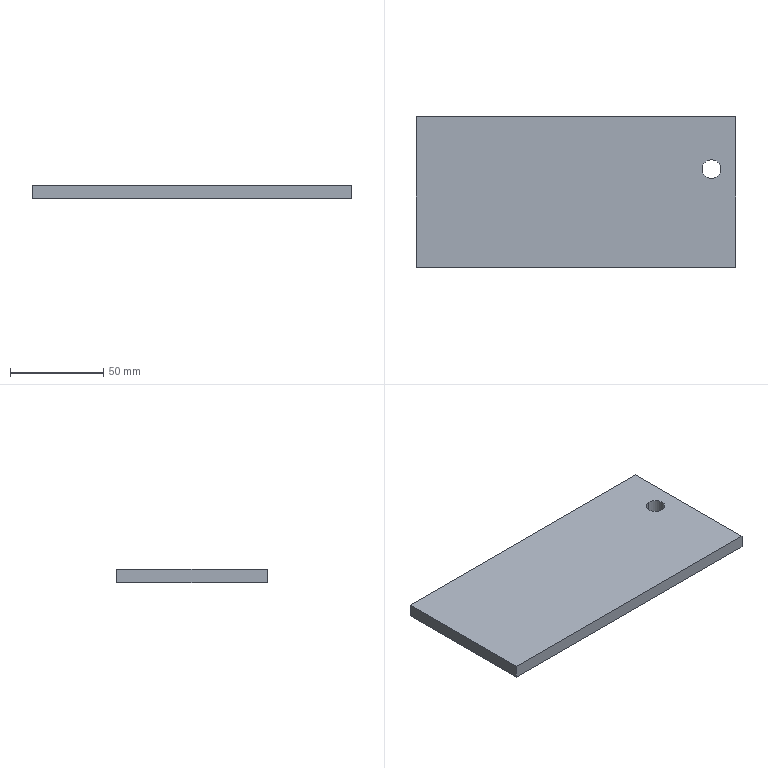Part | STEP file | 2026.6.15-Main Assembly图.sldasm-Part-138 | 1 solid | 8 faces | box 170.9 x 80.5 x 7 mm | volume 95752 mm3 | plane 6 | cylinder 2 | commonest cylinder face diameters 10 x2
STEP:
#1=CARTESIAN_POINT('',(-1516.724,576.551,4343.667));
#2=VERTEX_POINT('',#1);
#3=CARTESIAN_POINT('',(-1516.724,566.551,4343.667));
#4=VERTEX_POINT('',#3);
#5=CARTESIAN_POINT('',(-1516.724,571.551,4343.667));
#6=DIRECTION('',(0.,0.,1.));
#7=DIRECTION('',(0.,-1.,0.));
#8=AXIS2_PLACEMENT_3D('',#5,#6,#7);
#9=CIRCLE('',#8,5.);
#10=EDGE_CURVE('',#2,#4,#9,.T.);
#11=ORIENTED_EDGE('',*,*,#10,.T.);
#12=CARTESIAN_POINT('',(-1516.724,566.551,4336.667));
#13=VERTEX_POINT('',#12);
#14=CARTESIAN_POINT('',(-1516.724,566.551,4343.667));
#15=DIRECTION('',(0.,0.,-1.));
#16=VECTOR('',#15,1000.);
#17=LINE('',#14,#16);
#18=EDGE_CURVE('',#4,#13,#17,.T.);
#19=ORIENTED_EDGE('',*,*,#18,.T.);
#20=CARTESIAN_POINT('',(-1516.724,576.551,4336.667));
#21=VERTEX_POINT('',#20);
#22=CARTESIAN_POINT('',(-1516.724,571.551,4336.667));
#23=DIRECTION('',(0.,0.,1.));
#24=DIRECTION('',(0.,-1.,0.));
#25=AXIS2_PLACEMENT_3D('',#22,#23,#24);
#26=CIRCLE('',#25,5.);
#27=EDGE_CURVE('',#21,#13,#26,.T.);
#28=ORIENTED_EDGE('',*,*,#27,.F.);
#29=CARTESIAN_POINT('',(-1516.724,576.551,4343.667));
#30=DIRECTION('',(0.,0.,-1.));
#31=VECTOR('',#30,1000.);
#32=LINE('',#29,#31);
#33=EDGE_CURVE('',#2,#21,#32,.T.);
#34=ORIENTED_EDGE('',*,*,#33,.F.);
#35=EDGE_LOOP('',(#11,#19,#28,#34));
#36=FACE_OUTER_BOUND('',#35,.T.);
#37=CARTESIAN_POINT('',(-1516.724,571.551,4343.667));
#38=DIRECTION('',(0.,0.,-1.));
#39=DIRECTION('',(0.,1.,0.));
#40=AXIS2_PLACEMENT_3D('',#37,#38,#39);
#41=CYLINDRICAL_SURFACE('',#40,5.);
#42=ADVANCED_FACE('',(#36),#41,.F.);
#43=CARTESIAN_POINT('',(-1674.674,599.551,4336.667));
#44=VERTEX_POINT('',#43);
#45=CARTESIAN_POINT('',(-1674.674,519.051,4336.667));
#46=VERTEX_POINT('',#45);
#47=CARTESIAN_POINT('',(-1674.674,599.551,4336.667));
#48=DIRECTION('',(0.,-1.,0.));
#49=VECTOR('',#48,1000.);
#50=LINE('',#47,#49);
#51=EDGE_CURVE('',#44,#46,#50,.T.);
#52=ORIENTED_EDGE('',*,*,#51,.T.);
#53=CARTESIAN_POINT('',(-1674.674,519.051,4343.667));
#54=VERTEX_POINT('',#53);
#55=CARTESIAN_POINT('',(-1674.674,519.051,4343.667));
#56=DIRECTION('',(0.,0.,-1.));
#57=VECTOR('',#56,1000.);
#58=LINE('',#55,#57);
#59=EDGE_CURVE('',#54,#46,#58,.T.);
#60=ORIENTED_EDGE('',*,*,#59,.F.);
#61=CARTESIAN_POINT('',(-1674.674,599.551,4343.667));
#62=VERTEX_POINT('',#61);
#63=CARTESIAN_POINT('',(-1674.674,599.551,4343.667));
#64=DIRECTION('',(0.,-1.,0.));
#65=VECTOR('',#64,1000.);
#66=LINE('',#63,#65);
#67=EDGE_CURVE('',#62,#54,#66,.T.);
#68=ORIENTED_EDGE('',*,*,#67,.F.);
#69=CARTESIAN_POINT('',(-1674.674,599.551,4343.667));
#70=DIRECTION('',(0.,0.,-1.));
#71=VECTOR('',#70,1000.);
#72=LINE('',#69,#71);
#73=EDGE_CURVE('',#62,#44,#72,.T.);
#74=ORIENTED_EDGE('',*,*,#73,.T.);
#75=EDGE_LOOP('',(#52,#60,#68,#74));
#76=FACE_OUTER_BOUND('',#75,.T.);
#77=CARTESIAN_POINT('',(-1674.674,599.551,4343.667));
#78=DIRECTION('',(1.,0.,0.));
#79=DIRECTION('',(0.,1.,0.));
#80=AXIS2_PLACEMENT_3D('',#77,#78,#79);
#81=PLANE('',#80);
#82=ADVANCED_FACE('',(#76),#81,.F.);
#83=CARTESIAN_POINT('',(-1503.774,519.051,4336.667));
#84=VERTEX_POINT('',#83);
#85=CARTESIAN_POINT('',(-1674.674,519.051,4336.667));
#86=DIRECTION('',(1.,0.,0.));
#87=VECTOR('',#86,1000.);
#88=LINE('',#85,#87);
#89=EDGE_CURVE('',#46,#84,#88,.T.);
#90=ORIENTED_EDGE('',*,*,#89,.T.);
#91=CARTESIAN_POINT('',(-1503.774,519.051,4343.667));
#92=VERTEX_POINT('',#91);
#93=CARTESIAN_POINT('',(-1503.774,519.051,4343.667));
#94=DIRECTION('',(0.,0.,-1.));
#95=VECTOR('',#94,1000.);
#96=LINE('',#93,#95);
#97=EDGE_CURVE('',#92,#84,#96,.T.);
#98=ORIENTED_EDGE('',*,*,#97,.F.);
#99=CARTESIAN_POINT('',(-1674.674,519.051,4343.667));
#100=DIRECTION('',(1.,0.,0.));
#101=VECTOR('',#100,1000.);
#102=LINE('',#99,#101);
#103=EDGE_CURVE('',#54,#92,#102,.T.);
#104=ORIENTED_EDGE('',*,*,#103,.F.);
#105=ORIENTED_EDGE('',*,*,#59,.T.);
#106=EDGE_LOOP('',(#90,#98,#104,#105));
#107=FACE_OUTER_BOUND('',#106,.T.);
#108=CARTESIAN_POINT('',(-1674.674,519.051,4343.667));
#109=DIRECTION('',(0.,1.,0.));
#110=DIRECTION('',(0.,0.,1.));
#111=AXIS2_PLACEMENT_3D('',#108,#109,#110);
#112=PLANE('',#111);
#113=ADVANCED_FACE('',(#107),#112,.F.);
#114=CARTESIAN_POINT('',(-1503.774,599.551,4336.667));
#115=VERTEX_POINT('',#114);
#116=CARTESIAN_POINT('',(-1503.774,519.051,4336.667));
#117=DIRECTION('',(0.,1.,0.));
#118=VECTOR('',#117,1000.);
#119=LINE('',#116,#118);
#120=EDGE_CURVE('',#84,#115,#119,.T.);
#121=ORIENTED_EDGE('',*,*,#120,.T.);
#122=CARTESIAN_POINT('',(-1503.774,599.551,4343.667));
#123=VERTEX_POINT('',#122);
#124=CARTESIAN_POINT('',(-1503.774,599.551,4343.667));
#125=DIRECTION('',(0.,0.,-1.));
#126=VECTOR('',#125,1000.);
#127=LINE('',#124,#126);
#128=EDGE_CURVE('',#123,#115,#127,.T.);
#129=ORIENTED_EDGE('',*,*,#128,.F.);
#130=CARTESIAN_POINT('',(-1503.774,519.051,4343.667));
#131=DIRECTION('',(0.,1.,0.));
#132=VECTOR('',#131,1000.);
#133=LINE('',#130,#132);
#134=EDGE_CURVE('',#92,#123,#133,.T.);
#135=ORIENTED_EDGE('',*,*,#134,.F.);
#136=ORIENTED_EDGE('',*,*,#97,.T.);
#137=EDGE_LOOP('',(#121,#129,#135,#136));
#138=FACE_OUTER_BOUND('',#137,.T.);
#139=CARTESIAN_POINT('',(-1503.774,519.051,4343.667));
#140=DIRECTION('',(-1.,0.,0.));
#141=DIRECTION('',(0.,-1.,0.));
#142=AXIS2_PLACEMENT_3D('',#139,#140,#141);
#143=PLANE('',#142);
#144=ADVANCED_FACE('',(#138),#143,.F.);
#145=CARTESIAN_POINT('',(-1503.774,599.551,4336.667));
#146=DIRECTION('',(-1.,0.,0.));
#147=VECTOR('',#146,1000.);
#148=LINE('',#145,#147);
#149=EDGE_CURVE('',#115,#44,#148,.T.);
#150=ORIENTED_EDGE('',*,*,#149,.T.);
#151=ORIENTED_EDGE('',*,*,#73,.F.);
#152=CARTESIAN_POINT('',(-1503.774,599.551,4343.667));
#153=DIRECTION('',(-1.,0.,0.));
#154=VECTOR('',#153,1000.);
#155=LINE('',#152,#154);
#156=EDGE_CURVE('',#123,#62,#155,.T.);
#157=ORIENTED_EDGE('',*,*,#156,.F.);
#158=ORIENTED_EDGE('',*,*,#128,.T.);
#159=EDGE_LOOP('',(#150,#151,#157,#158));
#160=FACE_OUTER_BOUND('',#159,.T.);
#161=CARTESIAN_POINT('',(-1503.774,599.551,4343.667));
#162=DIRECTION('',(0.,-1.,0.));
#163=DIRECTION('',(0.,0.,-1.));
#164=AXIS2_PLACEMENT_3D('',#161,#162,#163);
#165=PLANE('',#164);
#166=ADVANCED_FACE('',(#160),#165,.F.);
#167=ORIENTED_EDGE('',*,*,#18,.F.);
#168=CARTESIAN_POINT('',(-1516.724,571.551,4343.667));
#169=DIRECTION('',(0.,0.,1.));
#170=DIRECTION('',(0.,-1.,0.));
#171=AXIS2_PLACEMENT_3D('',#168,#169,#170);
#172=CIRCLE('',#171,5.);
#173=EDGE_CURVE('',#4,#2,#172,.T.);
#174=ORIENTED_EDGE('',*,*,#173,.T.);
#175=ORIENTED_EDGE('',*,*,#33,.T.);
#176=CARTESIAN_POINT('',(-1516.724,571.551,4336.667));
#177=DIRECTION('',(0.,0.,1.));
#178=DIRECTION('',(0.,-1.,0.));
#179=AXIS2_PLACEMENT_3D('',#176,#177,#178);
#180=CIRCLE('',#179,5.);
#181=EDGE_CURVE('',#13,#21,#180,.T.);
#182=ORIENTED_EDGE('',*,*,#181,.F.);
#183=EDGE_LOOP('',(#167,#174,#175,#182));
#184=FACE_OUTER_BOUND('',#183,.T.);
#185=CARTESIAN_POINT('',(-1516.724,571.551,4343.667));
#186=DIRECTION('',(0.,0.,-1.));
#187=DIRECTION('',(0.,1.,0.));
#188=AXIS2_PLACEMENT_3D('',#185,#186,#187);
#189=CYLINDRICAL_SURFACE('',#188,5.);
#190=ADVANCED_FACE('',(#184),#189,.F.);
#191=ORIENTED_EDGE('',*,*,#67,.T.);
#192=ORIENTED_EDGE('',*,*,#103,.T.);
#193=ORIENTED_EDGE('',*,*,#134,.T.);
#194=ORIENTED_EDGE('',*,*,#156,.T.);
#195=EDGE_LOOP('',(#191,#192,#193,#194));
#196=FACE_OUTER_BOUND('',#195,.T.);
#197=ORIENTED_EDGE('',*,*,#10,.F.);
#198=ORIENTED_EDGE('',*,*,#173,.F.);
#199=EDGE_LOOP('',(#197,#198));
#200=FACE_BOUND('',#199,.T.);
#201=CARTESIAN_POINT('',(-1516.724,571.551,4343.667));
#202=DIRECTION('',(0.,0.,1.));
#203=DIRECTION('',(0.,-1.,0.));
#204=AXIS2_PLACEMENT_3D('',#201,#202,#203);
#205=PLANE('',#204);
#206=ADVANCED_FACE('',(#196,#200),#205,.T.);
#207=ORIENTED_EDGE('',*,*,#51,.F.);
#208=ORIENTED_EDGE('',*,*,#149,.F.);
#209=ORIENTED_EDGE('',*,*,#120,.F.);
#210=ORIENTED_EDGE('',*,*,#89,.F.);
#211=EDGE_LOOP('',(#207,#208,#209,#210));
#212=FACE_OUTER_BOUND('',#211,.T.);
#213=ORIENTED_EDGE('',*,*,#27,.T.);
#214=ORIENTED_EDGE('',*,*,#181,.T.);
#215=EDGE_LOOP('',(#213,#214));
#216=FACE_BOUND('',#215,.T.);
#217=CARTESIAN_POINT('',(-1516.724,571.551,4336.667));
#218=DIRECTION('',(0.,0.,1.));
#219=DIRECTION('',(0.,-1.,0.));
#220=AXIS2_PLACEMENT_3D('',#217,#218,#219);
#221=PLANE('',#220);
#222=ADVANCED_FACE('',(#212,#216),#221,.F.);
#223=CLOSED_SHELL('',(#42,#82,#113,#144,#166,#190,#206,#222));
#224=MANIFOLD_SOLID_BREP('',#223);
#225=CARTESIAN_POINT('',(0.,0.,0.));
#226=DIRECTION('',(0.,0.,1.));
#227=DIRECTION('',(1.,0.,0.));
#228=AXIS2_PLACEMENT_3D('',#225,#226,#227);
#229=(LENGTH_UNIT()NAMED_UNIT(*)SI_UNIT(.MILLI.,.METRE.));
#230=UNCERTAINTY_MEASURE_WITH_UNIT(LENGTH_MEASURE(0.00001),#229,'','');
#231=(NAMED_UNIT(*)PLANE_ANGLE_UNIT()SI_UNIT($,.RADIAN.));
#232=(NAMED_UNIT(*)SI_UNIT($,.STERADIAN.)SOLID_ANGLE_UNIT());
#233=(GEOMETRIC_REPRESENTATION_CONTEXT(3)GLOBAL_UNCERTAINTY_ASSIGNED_CONTEXT((#230))GLOBAL_UNIT_ASSIGNED_CONTEXT((#229,#231,#232))REPRESENTATION_CONTEXT('',''));
#234=ADVANCED_BREP_SHAPE_REPRESENTATION('',(#224,#228),#233);